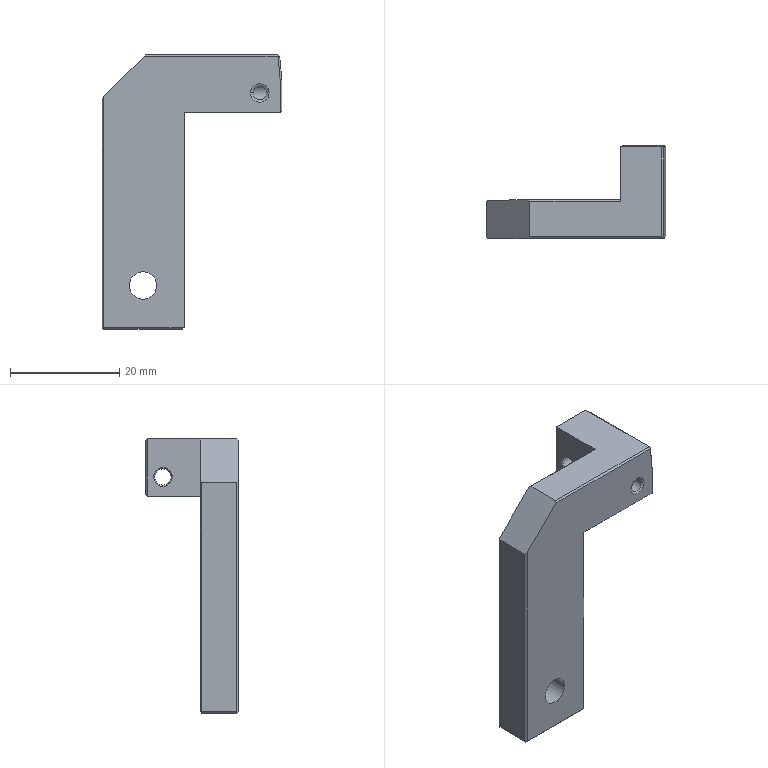Part | NX | 1 solid | 41 faces | box 32.9 x 17 x 50.2 mm | volume 6946 mm3 | plane 29 | cylinder 6 | cone 6 | commonest cylinder face diameters 2.5 x2 3 x2 5 x2